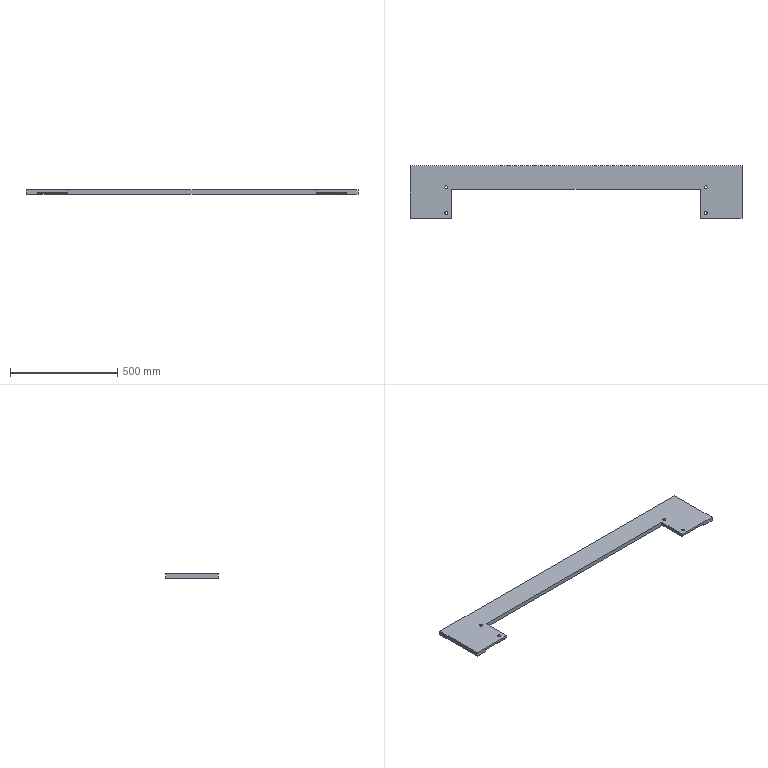Part | SolidWorks | features BaseBody 1 | 1 solid | 32 faces | box 1550 x 247 x 20 mm | volume 4227971 mm3 | plane 20 | cylinder 12 | commonest cylinder face diameters 14 x8 10 x4
STEP:
#1=CARTESIAN_POINT('',(612.,23.,20.));
#2=VERTEX_POINT('',#1);
#3=CARTESIAN_POINT('',(598.,23.,20.));
#4=VERTEX_POINT('',#3);
#5=CARTESIAN_POINT('',(605.,23.,20.));
#6=DIRECTION('',(0.,0.,-1.));
#7=DIRECTION('',(-1.,0.,0.));
#8=AXIS2_PLACEMENT_3D('',#5,#6,#7);
#9=CIRCLE('',#8,7.);
#10=EDGE_CURVE('',#2,#4,#9,.T.);
#11=ORIENTED_EDGE('',*,*,#10,.F.);
#12=CARTESIAN_POINT('',(612.,23.,5.));
#13=VERTEX_POINT('',#12);
#14=CARTESIAN_POINT('',(612.,23.,5.));
#15=DIRECTION('',(0.,0.,-1.));
#16=VECTOR('',#15,1000.);
#17=LINE('',#14,#16);
#18=EDGE_CURVE('',#2,#13,#17,.T.);
#19=ORIENTED_EDGE('',*,*,#18,.T.);
#20=CARTESIAN_POINT('',(598.,23.,5.));
#21=VERTEX_POINT('',#20);
#22=CARTESIAN_POINT('',(605.,23.,5.));
#23=DIRECTION('',(0.,0.,-1.));
#24=DIRECTION('',(-1.,0.,0.));
#25=AXIS2_PLACEMENT_3D('',#22,#23,#24);
#26=CIRCLE('',#25,7.);
#27=EDGE_CURVE('',#13,#21,#26,.T.);
#28=ORIENTED_EDGE('',*,*,#27,.T.);
#29=CARTESIAN_POINT('',(598.,23.,5.));
#30=DIRECTION('',(0.,0.,-1.));
#31=VECTOR('',#30,1000.);
#32=LINE('',#29,#31);
#33=EDGE_CURVE('',#4,#21,#32,.T.);
#34=ORIENTED_EDGE('',*,*,#33,.F.);
#35=EDGE_LOOP('',(#11,#19,#28,#34));
#36=FACE_OUTER_BOUND('',#35,.T.);
#37=CARTESIAN_POINT('',(605.,23.,5.));
#38=DIRECTION('',(0.,0.,-1.));
#39=DIRECTION('',(-1.,0.,0.));
#40=AXIS2_PLACEMENT_3D('',#37,#38,#39);
#41=CYLINDRICAL_SURFACE('',#40,7.);
#42=ADVANCED_FACE('',(#36),#41,.F.);
#43=CARTESIAN_POINT('',(612.,-97.,20.));
#44=VERTEX_POINT('',#43);
#45=CARTESIAN_POINT('',(598.,-97.,20.));
#46=VERTEX_POINT('',#45);
#47=CARTESIAN_POINT('',(605.,-97.,20.));
#48=DIRECTION('',(0.,0.,-1.));
#49=DIRECTION('',(-1.,0.,0.));
#50=AXIS2_PLACEMENT_3D('',#47,#48,#49);
#51=CIRCLE('',#50,7.);
#52=EDGE_CURVE('',#44,#46,#51,.T.);
#53=ORIENTED_EDGE('',*,*,#52,.F.);
#54=CARTESIAN_POINT('',(612.,-97.,5.));
#55=VERTEX_POINT('',#54);
#56=CARTESIAN_POINT('',(612.,-97.,5.));
#57=DIRECTION('',(0.,0.,-1.));
#58=VECTOR('',#57,1000.);
#59=LINE('',#56,#58);
#60=EDGE_CURVE('',#44,#55,#59,.T.);
#61=ORIENTED_EDGE('',*,*,#60,.T.);
#62=CARTESIAN_POINT('',(598.,-97.,5.));
#63=VERTEX_POINT('',#62);
#64=CARTESIAN_POINT('',(605.,-97.,5.));
#65=DIRECTION('',(0.,0.,-1.));
#66=DIRECTION('',(-1.,0.,0.));
#67=AXIS2_PLACEMENT_3D('',#64,#65,#66);
#68=CIRCLE('',#67,7.);
#69=EDGE_CURVE('',#55,#63,#68,.T.);
#70=ORIENTED_EDGE('',*,*,#69,.T.);
#71=CARTESIAN_POINT('',(598.,-97.,5.));
#72=DIRECTION('',(0.,0.,-1.));
#73=VECTOR('',#72,1000.);
#74=LINE('',#71,#73);
#75=EDGE_CURVE('',#46,#63,#74,.T.);
#76=ORIENTED_EDGE('',*,*,#75,.F.);
#77=EDGE_LOOP('',(#53,#61,#70,#76));
#78=FACE_OUTER_BOUND('',#77,.T.);
#79=CARTESIAN_POINT('',(605.,-97.,5.));
#80=DIRECTION('',(0.,0.,-1.));
#81=DIRECTION('',(-1.,0.,0.));
#82=AXIS2_PLACEMENT_3D('',#79,#80,#81);
#83=CYLINDRICAL_SURFACE('',#82,7.);
#84=ADVANCED_FACE('',(#78),#83,.F.);
#85=CARTESIAN_POINT('',(-598.,-97.,20.));
#86=VERTEX_POINT('',#85);
#87=CARTESIAN_POINT('',(-612.,-97.,20.));
#88=VERTEX_POINT('',#87);
#89=CARTESIAN_POINT('',(-605.,-97.,20.));
#90=DIRECTION('',(0.,0.,-1.));
#91=DIRECTION('',(-1.,0.,0.));
#92=AXIS2_PLACEMENT_3D('',#89,#90,#91);
#93=CIRCLE('',#92,7.);
#94=EDGE_CURVE('',#86,#88,#93,.T.);
#95=ORIENTED_EDGE('',*,*,#94,.F.);
#96=CARTESIAN_POINT('',(-598.,-97.,5.));
#97=VERTEX_POINT('',#96);
#98=CARTESIAN_POINT('',(-598.,-97.,5.));
#99=DIRECTION('',(0.,0.,-1.));
#100=VECTOR('',#99,1000.);
#101=LINE('',#98,#100);
#102=EDGE_CURVE('',#86,#97,#101,.T.);
#103=ORIENTED_EDGE('',*,*,#102,.T.);
#104=CARTESIAN_POINT('',(-612.,-97.,5.));
#105=VERTEX_POINT('',#104);
#106=CARTESIAN_POINT('',(-605.,-97.,5.));
#107=DIRECTION('',(0.,0.,-1.));
#108=DIRECTION('',(-1.,0.,0.));
#109=AXIS2_PLACEMENT_3D('',#106,#107,#108);
#110=CIRCLE('',#109,7.);
#111=EDGE_CURVE('',#97,#105,#110,.T.);
#112=ORIENTED_EDGE('',*,*,#111,.T.);
#113=CARTESIAN_POINT('',(-612.,-97.,5.));
#114=DIRECTION('',(0.,0.,-1.));
#115=VECTOR('',#114,1000.);
#116=LINE('',#113,#115);
#117=EDGE_CURVE('',#88,#105,#116,.T.);
#118=ORIENTED_EDGE('',*,*,#117,.F.);
#119=EDGE_LOOP('',(#95,#103,#112,#118));
#120=FACE_OUTER_BOUND('',#119,.T.);
#121=CARTESIAN_POINT('',(-605.,-97.,5.));
#122=DIRECTION('',(0.,0.,-1.));
#123=DIRECTION('',(-1.,0.,0.));
#124=AXIS2_PLACEMENT_3D('',#121,#122,#123);
#125=CYLINDRICAL_SURFACE('',#124,7.);
#126=ADVANCED_FACE('',(#120),#125,.F.);
#127=CARTESIAN_POINT('',(-598.,23.,20.));
#128=VERTEX_POINT('',#127);
#129=CARTESIAN_POINT('',(-612.,23.,20.));
#130=VERTEX_POINT('',#129);
#131=CARTESIAN_POINT('',(-605.,23.,20.));
#132=DIRECTION('',(0.,0.,-1.));
#133=DIRECTION('',(-1.,0.,0.));
#134=AXIS2_PLACEMENT_3D('',#131,#132,#133);
#135=CIRCLE('',#134,7.);
#136=EDGE_CURVE('',#128,#130,#135,.T.);
#137=ORIENTED_EDGE('',*,*,#136,.F.);
#138=CARTESIAN_POINT('',(-598.,23.,5.));
#139=VERTEX_POINT('',#138);
#140=CARTESIAN_POINT('',(-598.,23.,5.));
#141=DIRECTION('',(0.,0.,-1.));
#142=VECTOR('',#141,1000.);
#143=LINE('',#140,#142);
#144=EDGE_CURVE('',#128,#139,#143,.T.);
#145=ORIENTED_EDGE('',*,*,#144,.T.);
#146=CARTESIAN_POINT('',(-612.,23.,5.));
#147=VERTEX_POINT('',#146);
#148=CARTESIAN_POINT('',(-605.,23.,5.));
#149=DIRECTION('',(0.,0.,-1.));
#150=DIRECTION('',(-1.,0.,0.));
#151=AXIS2_PLACEMENT_3D('',#148,#149,#150);
#152=CIRCLE('',#151,7.);
#153=EDGE_CURVE('',#139,#147,#152,.T.);
#154=ORIENTED_EDGE('',*,*,#153,.T.);
#155=CARTESIAN_POINT('',(-612.,23.,5.));
#156=DIRECTION('',(0.,0.,-1.));
#157=VECTOR('',#156,1000.);
#158=LINE('',#155,#157);
#159=EDGE_CURVE('',#130,#147,#158,.T.);
#160=ORIENTED_EDGE('',*,*,#159,.F.);
#161=EDGE_LOOP('',(#137,#145,#154,#160));
#162=FACE_OUTER_BOUND('',#161,.T.);
#163=CARTESIAN_POINT('',(-605.,23.,5.));
#164=DIRECTION('',(0.,0.,-1.));
#165=DIRECTION('',(-1.,0.,0.));
#166=AXIS2_PLACEMENT_3D('',#163,#164,#165);
#167=CYLINDRICAL_SURFACE('',#166,7.);
#168=ADVANCED_FACE('',(#162),#167,.F.);
#169=CARTESIAN_POINT('',(580.,-117.,5.));
#170=VERTEX_POINT('',#169);
#171=CARTESIAN_POINT('',(580.,15.,5.));
#172=VERTEX_POINT('',#171);
#173=CARTESIAN_POINT('',(580.,-122.,5.));
#174=DIRECTION('',(0.,1.,0.));
#175=VECTOR('',#174,1000.);
#176=LINE('',#173,#175);
#177=EDGE_CURVE('',#170,#172,#176,.T.);
#178=ORIENTED_EDGE('',*,*,#177,.F.);
#179=CARTESIAN_POINT('',(580.,-122.,10.));
#180=VERTEX_POINT('',#179);
#181=CARTESIAN_POINT('',(580.,-117.,5.));
#182=DIRECTION('',(0.,-0.7071,0.7071));
#183=VECTOR('',#182,1000.);
#184=LINE('',#181,#183);
#185=EDGE_CURVE('',#170,#180,#184,.T.);
#186=ORIENTED_EDGE('',*,*,#185,.T.);
#187=CARTESIAN_POINT('',(580.,-122.,20.));
#188=VERTEX_POINT('',#187);
#189=CARTESIAN_POINT('',(580.,-122.,20.));
#190=DIRECTION('',(0.,0.,-1.));
#191=VECTOR('',#190,1000.);
#192=LINE('',#189,#191);
#193=EDGE_CURVE('',#188,#180,#192,.T.);
#194=ORIENTED_EDGE('',*,*,#193,.F.);
#195=CARTESIAN_POINT('',(580.,15.,20.));
#196=VERTEX_POINT('',#195);
#197=CARTESIAN_POINT('',(580.,15.,20.));
#198=DIRECTION('',(0.,-1.,0.));
#199=VECTOR('',#198,1000.);
#200=LINE('',#197,#199);
#201=EDGE_CURVE('',#196,#188,#200,.T.);
#202=ORIENTED_EDGE('',*,*,#201,.F.);
#203=CARTESIAN_POINT('',(580.,15.,20.));
#204=DIRECTION('',(0.,0.,-1.));
#205=VECTOR('',#204,1000.);
#206=LINE('',#203,#205);
#207=EDGE_CURVE('',#196,#172,#206,.T.);
#208=ORIENTED_EDGE('',*,*,#207,.T.);
#209=EDGE_LOOP('',(#178,#186,#194,#202,#208));
#210=FACE_OUTER_BOUND('',#209,.T.);
#211=CARTESIAN_POINT('',(580.,15.,20.));
#212=DIRECTION('',(1.,0.,0.));
#213=DIRECTION('',(0.,0.,-1.));
#214=AXIS2_PLACEMENT_3D('',#211,#212,#213);
#215=PLANE('',#214);
#216=ADVANCED_FACE('',(#210),#215,.F.);
#217=CARTESIAN_POINT('',(605.,23.,20.));
#218=DIRECTION('',(0.,0.,-1.));
#219=DIRECTION('',(-1.,0.,0.));
#220=AXIS2_PLACEMENT_3D('',#217,#218,#219);
#221=CIRCLE('',#220,7.);
#222=EDGE_CURVE('',#4,#2,#221,.T.);
#223=ORIENTED_EDGE('',*,*,#222,.T.);
#224=ORIENTED_EDGE('',*,*,#10,.T.);
#225=EDGE_LOOP('',(#223,#224));
#226=FACE_BOUND('',#225,.T.);
#227=CARTESIAN_POINT('',(605.,-97.,20.));
#228=DIRECTION('',(0.,0.,-1.));
#229=DIRECTION('',(-1.,0.,0.));
#230=AXIS2_PLACEMENT_3D('',#227,#228,#229);
#231=CIRCLE('',#230,7.);
#232=EDGE_CURVE('',#46,#44,#231,.T.);
#233=ORIENTED_EDGE('',*,*,#232,.T.);
#234=ORIENTED_EDGE('',*,*,#52,.T.);
#235=EDGE_LOOP('',(#233,#234));
#236=FACE_BOUND('',#235,.T.);
#237=CARTESIAN_POINT('',(-605.,-97.,20.));
#238=DIRECTION('',(0.,0.,-1.));
#239=DIRECTION('',(-1.,0.,0.));
#240=AXIS2_PLACEMENT_3D('',#237,#238,#239);
#241=CIRCLE('',#240,7.);
#242=EDGE_CURVE('',#88,#86,#241,.T.);
#243=ORIENTED_EDGE('',*,*,#242,.T.);
#244=ORIENTED_EDGE('',*,*,#94,.T.);
#245=EDGE_LOOP('',(#243,#244));
#246=FACE_BOUND('',#245,.T.);
#247=CARTESIAN_POINT('',(-605.,23.,20.));
#248=DIRECTION('',(0.,0.,-1.));
#249=DIRECTION('',(-1.,0.,0.));
#250=AXIS2_PLACEMENT_3D('',#247,#248,#249);
#251=CIRCLE('',#250,7.);
#252=EDGE_CURVE('',#130,#128,#251,.T.);
#253=ORIENTED_EDGE('',*,*,#252,.T.);
#254=ORIENTED_EDGE('',*,*,#136,.T.);
#255=EDGE_LOOP('',(#253,#254));
#256=FACE_BOUND('',#255,.T.);
#257=CARTESIAN_POINT('',(775.,-122.,20.));
#258=VERTEX_POINT('',#257);
#259=CARTESIAN_POINT('',(0.,-122.,20.));
#260=DIRECTION('',(-1.,0.,0.));
#261=VECTOR('',#260,1000.);
#262=LINE('',#259,#261);
#263=EDGE_CURVE('',#258,#188,#262,.T.);
#264=ORIENTED_EDGE('',*,*,#263,.F.);
#265=CARTESIAN_POINT('',(775.,125.,20.));
#266=VERTEX_POINT('',#265);
#267=CARTESIAN_POINT('',(775.,125.,20.));
#268=DIRECTION('',(0.,1.,0.));
#269=VECTOR('',#268,1000.);
#270=LINE('',#267,#269);
#271=EDGE_CURVE('',#258,#266,#270,.T.);
#272=ORIENTED_EDGE('',*,*,#271,.T.);
#273=CARTESIAN_POINT('',(-775.,125.,20.));
#274=VERTEX_POINT('',#273);
#275=CARTESIAN_POINT('',(-775.,125.,20.));
#276=DIRECTION('',(-1.,0.,0.));
#277=VECTOR('',#276,1000.);
#278=LINE('',#275,#277);
#279=EDGE_CURVE('',#266,#274,#278,.T.);
#280=ORIENTED_EDGE('',*,*,#279,.T.);
#281=CARTESIAN_POINT('',(-775.,-122.,20.));
#282=VERTEX_POINT('',#281);
#283=CARTESIAN_POINT('',(-775.,125.,20.));
#284=DIRECTION('',(0.,-1.,0.));
#285=VECTOR('',#284,1000.);
#286=LINE('',#283,#285);
#287=EDGE_CURVE('',#274,#282,#286,.T.);
#288=ORIENTED_EDGE('',*,*,#287,.T.);
#289=CARTESIAN_POINT('',(-580.,-122.,20.));
#290=VERTEX_POINT('',#289);
#291=CARTESIAN_POINT('',(0.,-122.,20.));
#292=DIRECTION('',(-1.,0.,0.));
#293=VECTOR('',#292,1000.);
#294=LINE('',#291,#293);
#295=EDGE_CURVE('',#290,#282,#294,.T.);
#296=ORIENTED_EDGE('',*,*,#295,.F.);
#297=CARTESIAN_POINT('',(-580.,15.,20.));
#298=VERTEX_POINT('',#297);
#299=CARTESIAN_POINT('',(-580.,15.,20.));
#300=DIRECTION('',(0.,1.,0.));
#301=VECTOR('',#300,1000.);
#302=LINE('',#299,#301);
#303=EDGE_CURVE('',#290,#298,#302,.T.);
#304=ORIENTED_EDGE('',*,*,#303,.T.);
#305=CARTESIAN_POINT('',(-580.,15.,20.));
#306=DIRECTION('',(1.,0.,0.));
#307=VECTOR('',#306,1000.);
#308=LINE('',#305,#307);
#309=EDGE_CURVE('',#298,#196,#308,.T.);
#310=ORIENTED_EDGE('',*,*,#309,.T.);
#311=ORIENTED_EDGE('',*,*,#201,.T.);
#312=EDGE_LOOP('',(#264,#272,#280,#288,#296,#304,#310,#311));
#313=FACE_OUTER_BOUND('',#312,.T.);
#314=CARTESIAN_POINT('',(0.,0.,20.));
#315=DIRECTION('',(0.,0.,-1.));
#316=DIRECTION('',(-1.,0.,0.));
#317=AXIS2_PLACEMENT_3D('',#314,#315,#316);
#318=PLANE('',#317);
#319=ADVANCED_FACE('',(#226,#236,#246,#256,#313),#318,.F.);
#320=CARTESIAN_POINT('',(-720.,-122.,0.));
#321=VERTEX_POINT('',#320);
#322=CARTESIAN_POINT('',(-720.,43.,0.));
#323=VERTEX_POINT('',#322);
#324=CARTESIAN_POINT('',(-720.,-122.,0.));
#325=DIRECTION('',(0.,1.,0.));
#326=VECTOR('',#325,1000.);
#327=LINE('',#324,#326);
#328=EDGE_CURVE('',#321,#323,#327,.T.);
#329=ORIENTED_EDGE('',*,*,#328,.F.);
#330=CARTESIAN_POINT('',(-775.,-122.,0.));
#331=VERTEX_POINT('',#330);
#332=CARTESIAN_POINT('',(-775.,-122.,0.));
#333=DIRECTION('',(1.,0.,0.));
#334=VECTOR('',#333,1000.);
#335=LINE('',#332,#334);
#336=EDGE_CURVE('',#331,#321,#335,.T.);
#337=ORIENTED_EDGE('',*,*,#336,.F.);
#338=CARTESIAN_POINT('',(-775.,125.,0.));
#339=VERTEX_POINT('',#338);
#340=CARTESIAN_POINT('',(-775.,125.,0.));
#341=DIRECTION('',(0.,-1.,0.));
#342=VECTOR('',#341,1000.);
#343=LINE('',#340,#342);
#344=EDGE_CURVE('',#339,#331,#343,.T.);
#345=ORIENTED_EDGE('',*,*,#344,.F.);
#346=CARTESIAN_POINT('',(775.,125.,0.));
#347=VERTEX_POINT('',#346);
#348=CARTESIAN_POINT('',(-775.,125.,0.));
#349=DIRECTION('',(-1.,0.,0.));
#350=VECTOR('',#349,1000.);
#351=LINE('',#348,#350);
#352=EDGE_CURVE('',#347,#339,#351,.T.);
#353=ORIENTED_EDGE('',*,*,#352,.F.);
#354=CARTESIAN_POINT('',(775.,-122.,0.));
#355=VERTEX_POINT('',#354);
#356=CARTESIAN_POINT('',(775.,125.,0.));
#357=DIRECTION('',(0.,1.,0.));
#358=VECTOR('',#357,1000.);
#359=LINE('',#356,#358);
#360=EDGE_CURVE('',#355,#347,#359,.T.);
#361=ORIENTED_EDGE('',*,*,#360,.F.);
#362=CARTESIAN_POINT('',(720.,-122.,0.));
#363=VERTEX_POINT('',#362);
#364=CARTESIAN_POINT('',(580.,-122.,0.));
#365=DIRECTION('',(1.,0.,0.));
#366=VECTOR('',#365,1000.);
#367=LINE('',#364,#366);
#368=EDGE_CURVE('',#363,#355,#367,.T.);
#369=ORIENTED_EDGE('',*,*,#368,.F.);
#370=CARTESIAN_POINT('',(720.,43.,0.));
#371=VERTEX_POINT('',#370);
#372=CARTESIAN_POINT('',(720.,-122.,0.));
#373=DIRECTION('',(0.,-1.,0.));
#374=VECTOR('',#373,1000.);
#375=LINE('',#372,#374);
#376=EDGE_CURVE('',#371,#363,#375,.T.);
#377=ORIENTED_EDGE('',*,*,#376,.F.);
#378=CARTESIAN_POINT('',(715.,48.,0.));
#379=VERTEX_POINT('',#378);
#380=CARTESIAN_POINT('',(715.,43.,0.));
#381=DIRECTION('',(0.,0.,-1.));
#382=DIRECTION('',(-1.,0.,0.));
#383=AXIS2_PLACEMENT_3D('',#380,#381,#382);
#384=CIRCLE('',#383,5.);
#385=EDGE_CURVE('',#379,#371,#384,.T.);
#386=ORIENTED_EDGE('',*,*,#385,.F.);
#387=CARTESIAN_POINT('',(585.,48.,0.));
#388=VERTEX_POINT('',#387);
#389=CARTESIAN_POINT('',(585.,48.,0.));
#390=DIRECTION('',(1.,0.,0.));
#391=VECTOR('',#390,1000.);
#392=LINE('',#389,#391);
#393=EDGE_CURVE('',#388,#379,#392,.T.);
#394=ORIENTED_EDGE('',*,*,#393,.F.);
#395=CARTESIAN_POINT('',(580.,43.,0.));
#396=VERTEX_POINT('',#395);
#397=CARTESIAN_POINT('',(585.,43.,0.));
#398=DIRECTION('',(0.,0.,-1.));
#399=DIRECTION('',(-1.,0.,0.));
#400=AXIS2_PLACEMENT_3D('',#397,#398,#399);
#401=CIRCLE('',#400,5.);
#402=EDGE_CURVE('',#396,#388,#401,.T.);
#403=ORIENTED_EDGE('',*,*,#402,.F.);
#404=CARTESIAN_POINT('',(580.,15.,0.));
#405=VERTEX_POINT('',#404);
#406=CARTESIAN_POINT('',(580.,-122.,0.));
#407=DIRECTION('',(0.,1.,0.));
#408=VECTOR('',#407,1000.);
#409=LINE('',#406,#408);
#410=EDGE_CURVE('',#405,#396,#409,.T.);
#411=ORIENTED_EDGE('',*,*,#410,.F.);
#412=CARTESIAN_POINT('',(-580.,15.,0.));
#413=VERTEX_POINT('',#412);
#414=CARTESIAN_POINT('',(-580.,15.,0.));
#415=DIRECTION('',(1.,0.,0.));
#416=VECTOR('',#415,1000.);
#417=LINE('',#414,#416);
#418=EDGE_CURVE('',#413,#405,#417,.T.);
#419=ORIENTED_EDGE('',*,*,#418,.F.);
#420=CARTESIAN_POINT('',(-580.,43.,0.));
#421=VERTEX_POINT('',#420);
#422=CARTESIAN_POINT('',(-580.,-122.,0.));
#423=DIRECTION('',(0.,-1.,0.));
#424=VECTOR('',#423,1000.);
#425=LINE('',#422,#424);
#426=EDGE_CURVE('',#421,#413,#425,.T.);
#427=ORIENTED_EDGE('',*,*,#426,.F.);
#428=CARTESIAN_POINT('',(-585.,48.,0.));
#429=VERTEX_POINT('',#428);
#430=CARTESIAN_POINT('',(-585.,43.,0.));
#431=DIRECTION('',(0.,0.,-1.));
#432=DIRECTION('',(1.,0.,0.));
#433=AXIS2_PLACEMENT_3D('',#430,#431,#432);
#434=CIRCLE('',#433,5.);
#435=EDGE_CURVE('',#429,#421,#434,.T.);
#436=ORIENTED_EDGE('',*,*,#435,.F.);
#437=CARTESIAN_POINT('',(-715.,48.,0.));
#438=VERTEX_POINT('',#437);
#439=CARTESIAN_POINT('',(-585.,48.,0.));
#440=DIRECTION('',(1.,0.,0.));
#441=VECTOR('',#440,1000.);
#442=LINE('',#439,#441);
#443=EDGE_CURVE('',#438,#429,#442,.T.);
#444=ORIENTED_EDGE('',*,*,#443,.F.);
#445=CARTESIAN_POINT('',(-715.,43.,0.));
#446=DIRECTION('',(0.,0.,-1.));
#447=DIRECTION('',(1.,0.,0.));
#448=AXIS2_PLACEMENT_3D('',#445,#446,#447);
#449=CIRCLE('',#448,5.);
#450=EDGE_CURVE('',#323,#438,#449,.T.);
#451=ORIENTED_EDGE('',*,*,#450,.F.);
#452=EDGE_LOOP('',(#329,#337,#345,#353,#361,#369,#377,#386,#394,#403,#411,#419,#427,#436,#444,#451));
#453=FACE_OUTER_BOUND('',#452,.T.);
#454=CARTESIAN_POINT('',(0.,0.,0.));
#455=DIRECTION('',(0.,0.,-1.));
#456=DIRECTION('',(-1.,0.,0.));
#457=AXIS2_PLACEMENT_3D('',#454,#455,#456);
#458=PLANE('',#457);
#459=ADVANCED_FACE('',(#453),#458,.T.);
#460=CARTESIAN_POINT('',(775.,-122.,170.));
#461=DIRECTION('',(0.,0.,1.));
#462=VECTOR('',#461,1000.);
#463=LINE('',#460,#462);
#464=EDGE_CURVE('',#355,#258,#463,.T.);
#465=ORIENTED_EDGE('',*,*,#464,.F.);
#466=ORIENTED_EDGE('',*,*,#360,.T.);
#467=CARTESIAN_POINT('',(775.,125.,20.));
#468=DIRECTION('',(0.,0.,-1.));
#469=VECTOR('',#468,1000.);
#470=LINE('',#467,#469);
#471=EDGE_CURVE('',#266,#347,#470,.T.);
#472=ORIENTED_EDGE('',*,*,#471,.F.);
#473=ORIENTED_EDGE('',*,*,#271,.F.);
#474=EDGE_LOOP('',(#465,#466,#472,#473));
#475=FACE_OUTER_BOUND('',#474,.T.);
#476=CARTESIAN_POINT('',(775.,125.,20.));
#477=DIRECTION('',(-1.,0.,0.));
#478=DIRECTION('',(0.,0.,1.));
#479=AXIS2_PLACEMENT_3D('',#476,#477,#478);
#480=PLANE('',#479);
#481=ADVANCED_FACE('',(#475),#480,.F.);
#482=CARTESIAN_POINT('',(-775.,-122.,170.));
#483=DIRECTION('',(0.,0.,-1.));
#484=VECTOR('',#483,1000.);
#485=LINE('',#482,#484);
#486=EDGE_CURVE('',#282,#331,#485,.T.);
#487=ORIENTED_EDGE('',*,*,#486,.F.);
#488=ORIENTED_EDGE('',*,*,#287,.F.);
#489=CARTESIAN_POINT('',(-775.,125.,20.));
#490=DIRECTION('',(0.,0.,-1.));
#491=VECTOR('',#490,1000.);
#492=LINE('',#489,#491);
#493=EDGE_CURVE('',#274,#339,#492,.T.);
#494=ORIENTED_EDGE('',*,*,#493,.T.);
#495=ORIENTED_EDGE('',*,*,#344,.T.);
#496=EDGE_LOOP('',(#487,#488,#494,#495));
#497=FACE_OUTER_BOUND('',#496,.T.);
#498=CARTESIAN_POINT('',(-775.,125.,20.));
#499=DIRECTION('',(1.,0.,0.));
#500=DIRECTION('',(0.,0.,-1.));
#501=AXIS2_PLACEMENT_3D('',#498,#499,#500);
#502=PLANE('',#501);
#503=ADVANCED_FACE('',(#497),#502,.F.);
#504=CARTESIAN_POINT('',(-580.,-122.,10.));
#505=VERTEX_POINT('',#504);
#506=CARTESIAN_POINT('',(-580.,-122.,170.));
#507=DIRECTION('',(0.,0.,1.));
#508=VECTOR('',#507,1000.);
#509=LINE('',#506,#508);
#510=EDGE_CURVE('',#505,#290,#509,.T.);
#511=ORIENTED_EDGE('',*,*,#510,.F.);
#512=CARTESIAN_POINT('',(-580.,-117.,5.));
#513=VERTEX_POINT('',#512);
#514=CARTESIAN_POINT('',(-580.,-117.,5.));
#515=DIRECTION('',(0.,0.7071,-0.7071));
#516=VECTOR('',#515,1000.);
#517=LINE('',#514,#516);
#518=EDGE_CURVE('',#505,#513,#517,.T.);
#519=ORIENTED_EDGE('',*,*,#518,.T.);
#520=CARTESIAN_POINT('',(-580.,15.,5.));
#521=VERTEX_POINT('',#520);
#522=CARTESIAN_POINT('',(-580.,-122.,5.));
#523=DIRECTION('',(0.,-1.,0.));
#524=VECTOR('',#523,1000.);
#525=LINE('',#522,#524);
#526=EDGE_CURVE('',#521,#513,#525,.T.);
#527=ORIENTED_EDGE('',*,*,#526,.F.);
#528=CARTESIAN_POINT('',(-580.,15.,20.));
#529=DIRECTION('',(0.,0.,-1.));
#530=VECTOR('',#529,1000.);
#531=LINE('',#528,#530);
#532=EDGE_CURVE('',#298,#521,#531,.T.);
#533=ORIENTED_EDGE('',*,*,#532,.F.);
#534=ORIENTED_EDGE('',*,*,#303,.F.);
#535=EDGE_LOOP('',(#511,#519,#527,#533,#534));
#536=FACE_OUTER_BOUND('',#535,.T.);
#537=CARTESIAN_POINT('',(-580.,15.,20.));
#538=DIRECTION('',(-1.,0.,0.));
#539=DIRECTION('',(0.,0.,1.));
#540=AXIS2_PLACEMENT_3D('',#537,#538,#539);
#541=PLANE('',#540);
#542=ADVANCED_FACE('',(#536),#541,.F.);
#543=ORIENTED_EDGE('',*,*,#352,.T.);
#544=ORIENTED_EDGE('',*,*,#493,.F.);
#545=ORIENTED_EDGE('',*,*,#279,.F.);
#546=ORIENTED_EDGE('',*,*,#471,.T.);
#547=EDGE_LOOP('',(#543,#544,#545,#546));
#548=FACE_OUTER_BOUND('',#547,.T.);
#549=CARTESIAN_POINT('',(-775.,125.,20.));
#550=DIRECTION('',(0.,-1.,0.));
#551=DIRECTION('',(0.,0.,-1.));
#552=AXIS2_PLACEMENT_3D('',#549,#550,#551);
#553=PLANE('',#552);
#554=ADVANCED_FACE('',(#548),#553,.F.);
#555=ORIENTED_EDGE('',*,*,#418,.T.);
#556=CARTESIAN_POINT('',(580.,15.,20.));
#557=DIRECTION('',(0.,0.,1.));
#558=VECTOR('',#557,1000.);
#559=LINE('',#556,#558);
#560=EDGE_CURVE('',#405,#172,#559,.T.);
#561=ORIENTED_EDGE('',*,*,#560,.T.);
#562=ORIENTED_EDGE('',*,*,#207,.F.);
#563=ORIENTED_EDGE('',*,*,#309,.F.);
#564=ORIENTED_EDGE('',*,*,#532,.T.);
#565=CARTESIAN_POINT('',(-580.,15.,20.));
#566=DIRECTION('',(0.,0.,-1.));
#567=VECTOR('',#566,1000.);
#568=LINE('',#565,#567);
#569=EDGE_CURVE('',#521,#413,#568,.T.);
#570=ORIENTED_EDGE('',*,*,#569,.T.);
#571=EDGE_LOOP('',(#555,#561,#562,#563,#564,#570));
#572=FACE_OUTER_BOUND('',#571,.T.);
#573=CARTESIAN_POINT('',(-580.,15.,20.));
#574=DIRECTION('',(0.,1.,0.));
#575=DIRECTION('',(0.,0.,1.));
#576=AXIS2_PLACEMENT_3D('',#573,#574,#575);
#577=PLANE('',#576);
#578=ADVANCED_FACE('',(#572),#577,.F.);
#579=CARTESIAN_POINT('',(-720.,-122.,10.));
#580=VERTEX_POINT('',#579);
#581=CARTESIAN_POINT('',(-720.,-122.,5.));
#582=DIRECTION('',(0.,0.,-1.));
#583=VECTOR('',#582,1000.);
#584=LINE('',#581,#583);
#585=EDGE_CURVE('',#580,#321,#584,.T.);
#586=ORIENTED_EDGE('',*,*,#585,.F.);
#587=CARTESIAN_POINT('',(-580.,-122.,10.));
#588=DIRECTION('',(1.,0.,0.));
#589=VECTOR('',#588,1000.);
#590=LINE('',#587,#589);
#591=EDGE_CURVE('',#580,#505,#590,.T.);
#592=ORIENTED_EDGE('',*,*,#591,.T.);
#593=ORIENTED_EDGE('',*,*,#510,.T.);
#594=ORIENTED_EDGE('',*,*,#295,.T.);
#595=ORIENTED_EDGE('',*,*,#486,.T.);
#596=ORIENTED_EDGE('',*,*,#336,.T.);
#597=EDGE_LOOP('',(#586,#592,#593,#594,#595,#596));
#598=FACE_OUTER_BOUND('',#597,.T.);
#599=CARTESIAN_POINT('',(0.,-122.,85.));
#600=DIRECTION('',(0.,-1.,0.));
#601=DIRECTION('',(0.,0.,-1.));
#602=AXIS2_PLACEMENT_3D('',#599,#600,#601);
#603=PLANE('',#602);
#604=ADVANCED_FACE('',(#598),#603,.T.);
#605=ORIENTED_EDGE('',*,*,#193,.T.);
#606=CARTESIAN_POINT('',(720.,-122.,10.));
#607=VERTEX_POINT('',#606);
#608=CARTESIAN_POINT('',(0.,-122.,10.));
#609=DIRECTION('',(1.,0.,0.));
#610=VECTOR('',#609,1000.);
#611=LINE('',#608,#610);
#612=EDGE_CURVE('',#180,#607,#611,.T.);
#613=ORIENTED_EDGE('',*,*,#612,.T.);
#614=CARTESIAN_POINT('',(720.,-122.,5.));
#615=DIRECTION('',(0.,0.,-1.));
#616=VECTOR('',#615,1000.);
#617=LINE('',#614,#616);
#618=EDGE_CURVE('',#607,#363,#617,.T.);
#619=ORIENTED_EDGE('',*,*,#618,.T.);
#620=ORIENTED_EDGE('',*,*,#368,.T.);
#621=ORIENTED_EDGE('',*,*,#464,.T.);
#622=ORIENTED_EDGE('',*,*,#263,.T.);
#623=EDGE_LOOP('',(#605,#613,#619,#620,#621,#622));
#624=FACE_OUTER_BOUND('',#623,.T.);
#625=CARTESIAN_POINT('',(0.,-122.,85.));
#626=DIRECTION('',(0.,-1.,0.));
#627=DIRECTION('',(0.,0.,-1.));
#628=AXIS2_PLACEMENT_3D('',#625,#626,#627);
#629=PLANE('',#628);
#630=ADVANCED_FACE('',(#624),#629,.T.);
#631=ORIENTED_EDGE('',*,*,#410,.T.);
#632=CARTESIAN_POINT('',(580.,43.,5.));
#633=VERTEX_POINT('',#632);
#634=CARTESIAN_POINT('',(580.,43.,5.));
#635=DIRECTION('',(0.,0.,-1.));
#636=VECTOR('',#635,1000.);
#637=LINE('',#634,#636);
#638=EDGE_CURVE('',#633,#396,#637,.T.);
#639=ORIENTED_EDGE('',*,*,#638,.F.);
#640=CARTESIAN_POINT('',(580.,-122.,5.));
#641=DIRECTION('',(0.,1.,0.));
#642=VECTOR('',#641,1000.);
#643=LINE('',#640,#642);
#644=EDGE_CURVE('',#172,#633,#643,.T.);
#645=ORIENTED_EDGE('',*,*,#644,.F.);
#646=ORIENTED_EDGE('',*,*,#560,.F.);
#647=EDGE_LOOP('',(#631,#639,#645,#646));
#648=FACE_OUTER_BOUND('',#647,.T.);
#649=CARTESIAN_POINT('',(580.,-122.,5.));
#650=DIRECTION('',(-1.,0.,0.));
#651=DIRECTION('',(0.,0.,1.));
#652=AXIS2_PLACEMENT_3D('',#649,#650,#651);
#653=PLANE('',#652);
#654=ADVANCED_FACE('',(#648),#653,.F.);
#655=ORIENTED_EDGE('',*,*,#376,.T.);
#656=ORIENTED_EDGE('',*,*,#618,.F.);
#657=CARTESIAN_POINT('',(720.,-117.,5.));
#658=VERTEX_POINT('',#657);
#659=CARTESIAN_POINT('',(720.,-119.5,7.5));
#660=DIRECTION('',(0.,0.7071,-0.7071));
#661=VECTOR('',#660,1000.);
#662=LINE('',#659,#661);
#663=EDGE_CURVE('',#607,#658,#662,.T.);
#664=ORIENTED_EDGE('',*,*,#663,.T.);
#665=CARTESIAN_POINT('',(720.,43.,5.));
#666=VERTEX_POINT('',#665);
#667=CARTESIAN_POINT('',(720.,-122.,5.));
#668=DIRECTION('',(0.,-1.,0.));
#669=VECTOR('',#668,1000.);
#670=LINE('',#667,#669);
#671=EDGE_CURVE('',#666,#658,#670,.T.);
#672=ORIENTED_EDGE('',*,*,#671,.F.);
#673=CARTESIAN_POINT('',(720.,43.,5.));
#674=DIRECTION('',(0.,0.,-1.));
#675=VECTOR('',#674,1000.);
#676=LINE('',#673,#675);
#677=EDGE_CURVE('',#666,#371,#676,.T.);
#678=ORIENTED_EDGE('',*,*,#677,.T.);
#679=EDGE_LOOP('',(#655,#656,#664,#672,#678));
#680=FACE_OUTER_BOUND('',#679,.T.);
#681=CARTESIAN_POINT('',(720.,-122.,5.));
#682=DIRECTION('',(1.,0.,0.));
#683=DIRECTION('',(0.,0.,-1.));
#684=AXIS2_PLACEMENT_3D('',#681,#682,#683);
#685=PLANE('',#684);
#686=ADVANCED_FACE('',(#680),#685,.F.);
#687=ORIENTED_EDGE('',*,*,#385,.T.);
#688=ORIENTED_EDGE('',*,*,#677,.F.);
#689=CARTESIAN_POINT('',(715.,48.,5.));
#690=VERTEX_POINT('',#689);
#691=CARTESIAN_POINT('',(715.,43.,5.));
#692=DIRECTION('',(0.,0.,-1.));
#693=DIRECTION('',(-1.,0.,0.));
#694=AXIS2_PLACEMENT_3D('',#691,#692,#693);
#695=CIRCLE('',#694,5.);
#696=EDGE_CURVE('',#690,#666,#695,.T.);
#697=ORIENTED_EDGE('',*,*,#696,.F.);
#698=CARTESIAN_POINT('',(715.,48.,5.));
#699=DIRECTION('',(0.,0.,-1.));
#700=VECTOR('',#699,1000.);
#701=LINE('',#698,#700);
#702=EDGE_CURVE('',#690,#379,#701,.T.);
#703=ORIENTED_EDGE('',*,*,#702,.T.);
#704=EDGE_LOOP('',(#687,#688,#697,#703));
#705=FACE_OUTER_BOUND('',#704,.T.);
#706=CARTESIAN_POINT('',(715.,43.,5.));
#707=DIRECTION('',(0.,0.,-1.));
#708=DIRECTION('',(-1.,0.,0.));
#709=AXIS2_PLACEMENT_3D('',#706,#707,#708);
#710=CYLINDRICAL_SURFACE('',#709,5.);
#711=ADVANCED_FACE('',(#705),#710,.F.);
#712=ORIENTED_EDGE('',*,*,#393,.T.);
#713=ORIENTED_EDGE('',*,*,#702,.F.);
#714=CARTESIAN_POINT('',(585.,48.,5.));
#715=VERTEX_POINT('',#714);
#716=CARTESIAN_POINT('',(585.,48.,5.));
#717=DIRECTION('',(1.,0.,0.));
#718=VECTOR('',#717,1000.);
#719=LINE('',#716,#718);
#720=EDGE_CURVE('',#715,#690,#719,.T.);
#721=ORIENTED_EDGE('',*,*,#720,.F.);
#722=CARTESIAN_POINT('',(585.,48.,5.));
#723=DIRECTION('',(0.,0.,-1.));
#724=VECTOR('',#723,1000.);
#725=LINE('',#722,#724);
#726=EDGE_CURVE('',#715,#388,#725,.T.);
#727=ORIENTED_EDGE('',*,*,#726,.T.);
#728=EDGE_LOOP('',(#712,#713,#721,#727));
#729=FACE_OUTER_BOUND('',#728,.T.);
#730=CARTESIAN_POINT('',(585.,48.,5.));
#731=DIRECTION('',(0.,1.,0.));
#732=DIRECTION('',(-1.,0.,0.));
#733=AXIS2_PLACEMENT_3D('',#730,#731,#732);
#734=PLANE('',#733);
#735=ADVANCED_FACE('',(#729),#734,.F.);
#736=ORIENTED_EDGE('',*,*,#402,.T.);
#737=ORIENTED_EDGE('',*,*,#726,.F.);
#738=CARTESIAN_POINT('',(585.,43.,5.));
#739=DIRECTION('',(0.,0.,-1.));
#740=DIRECTION('',(-1.,0.,0.));
#741=AXIS2_PLACEMENT_3D('',#738,#739,#740);
#742=CIRCLE('',#741,5.);
#743=EDGE_CURVE('',#633,#715,#742,.T.);
#744=ORIENTED_EDGE('',*,*,#743,.F.);
#745=ORIENTED_EDGE('',*,*,#638,.T.);
#746=EDGE_LOOP('',(#736,#737,#744,#745));
#747=FACE_OUTER_BOUND('',#746,.T.);
#748=CARTESIAN_POINT('',(585.,43.,5.));
#749=DIRECTION('',(0.,0.,-1.));
#750=DIRECTION('',(-1.,0.,0.));
#751=AXIS2_PLACEMENT_3D('',#748,#749,#750);
#752=CYLINDRICAL_SURFACE('',#751,5.);
#753=ADVANCED_FACE('',(#747),#752,.F.);
#754=CARTESIAN_POINT('',(605.,23.,5.));
#755=DIRECTION('',(0.,0.,-1.));
#756=DIRECTION('',(-1.,0.,0.));
#757=AXIS2_PLACEMENT_3D('',#754,#755,#756);
#758=CIRCLE('',#757,7.);
#759=EDGE_CURVE('',#21,#13,#758,.T.);
#760=ORIENTED_EDGE('',*,*,#759,.F.);
#761=ORIENTED_EDGE('',*,*,#27,.F.);
#762=EDGE_LOOP('',(#760,#761));
#763=FACE_BOUND('',#762,.T.);
#764=CARTESIAN_POINT('',(605.,-97.,5.));
#765=DIRECTION('',(0.,0.,-1.));
#766=DIRECTION('',(-1.,0.,0.));
#767=AXIS2_PLACEMENT_3D('',#764,#765,#766);
#768=CIRCLE('',#767,7.);
#769=EDGE_CURVE('',#63,#55,#768,.T.);
#770=ORIENTED_EDGE('',*,*,#769,.F.);
#771=ORIENTED_EDGE('',*,*,#69,.F.);
#772=EDGE_LOOP('',(#770,#771));
#773=FACE_BOUND('',#772,.T.);
#774=ORIENTED_EDGE('',*,*,#671,.T.);
#775=CARTESIAN_POINT('',(585.,-117.,5.));
#776=DIRECTION('',(-1.,0.,0.));
#777=VECTOR('',#776,1000.);
#778=LINE('',#775,#777);
#779=EDGE_CURVE('',#658,#170,#778,.T.);
#780=ORIENTED_EDGE('',*,*,#779,.T.);
#781=ORIENTED_EDGE('',*,*,#177,.T.);
#782=ORIENTED_EDGE('',*,*,#644,.T.);
#783=ORIENTED_EDGE('',*,*,#743,.T.);
#784=ORIENTED_EDGE('',*,*,#720,.T.);
#785=ORIENTED_EDGE('',*,*,#696,.T.);
#786=EDGE_LOOP('',(#774,#780,#781,#782,#783,#784,#785));
#787=FACE_OUTER_BOUND('',#786,.T.);
#788=CARTESIAN_POINT('',(585.,43.,5.));
#789=DIRECTION('',(0.,0.,-1.));
#790=DIRECTION('',(-1.,0.,0.));
#791=AXIS2_PLACEMENT_3D('',#788,#789,#790);
#792=PLANE('',#791);
#793=ADVANCED_FACE('',(#763,#773,#787),#792,.T.);
#794=CARTESIAN_POINT('',(-580.,43.,5.));
#795=VERTEX_POINT('',#794);
#796=CARTESIAN_POINT('',(-580.,-122.,5.));
#797=DIRECTION('',(0.,-1.,0.));
#798=VECTOR('',#797,1000.);
#799=LINE('',#796,#798);
#800=EDGE_CURVE('',#795,#521,#799,.T.);
#801=ORIENTED_EDGE('',*,*,#800,.F.);
#802=CARTESIAN_POINT('',(-580.,43.,5.));
#803=DIRECTION('',(0.,0.,-1.));
#804=VECTOR('',#803,1000.);
#805=LINE('',#802,#804);
#806=EDGE_CURVE('',#795,#421,#805,.T.);
#807=ORIENTED_EDGE('',*,*,#806,.T.);
#808=ORIENTED_EDGE('',*,*,#426,.T.);
#809=ORIENTED_EDGE('',*,*,#569,.F.);
#810=EDGE_LOOP('',(#801,#807,#808,#809));
#811=FACE_OUTER_BOUND('',#810,.T.);
#812=CARTESIAN_POINT('',(-580.,-122.,5.));
#813=DIRECTION('',(1.,0.,0.));
#814=DIRECTION('',(0.,0.,-1.));
#815=AXIS2_PLACEMENT_3D('',#812,#813,#814);
#816=PLANE('',#815);
#817=ADVANCED_FACE('',(#811),#816,.F.);
#818=ORIENTED_EDGE('',*,*,#450,.T.);
#819=CARTESIAN_POINT('',(-715.,48.,5.));
#820=VERTEX_POINT('',#819);
#821=CARTESIAN_POINT('',(-715.,48.,5.));
#822=DIRECTION('',(0.,0.,-1.));
#823=VECTOR('',#822,1000.);
#824=LINE('',#821,#823);
#825=EDGE_CURVE('',#820,#438,#824,.T.);
#826=ORIENTED_EDGE('',*,*,#825,.F.);
#827=CARTESIAN_POINT('',(-720.,43.,5.));
#828=VERTEX_POINT('',#827);
#829=CARTESIAN_POINT('',(-715.,43.,5.));
#830=DIRECTION('',(0.,0.,-1.));
#831=DIRECTION('',(1.,0.,0.));
#832=AXIS2_PLACEMENT_3D('',#829,#830,#831);
#833=CIRCLE('',#832,5.);
#834=EDGE_CURVE('',#828,#820,#833,.T.);
#835=ORIENTED_EDGE('',*,*,#834,.F.);
#836=CARTESIAN_POINT('',(-720.,43.,5.));
#837=DIRECTION('',(0.,0.,-1.));
#838=VECTOR('',#837,1000.);
#839=LINE('',#836,#838);
#840=EDGE_CURVE('',#828,#323,#839,.T.);
#841=ORIENTED_EDGE('',*,*,#840,.T.);
#842=EDGE_LOOP('',(#818,#826,#835,#841));
#843=FACE_OUTER_BOUND('',#842,.T.);
#844=CARTESIAN_POINT('',(-715.,43.,5.));
#845=DIRECTION('',(0.,0.,-1.));
#846=DIRECTION('',(-1.,0.,0.));
#847=AXIS2_PLACEMENT_3D('',#844,#845,#846);
#848=CYLINDRICAL_SURFACE('',#847,5.);
#849=ADVANCED_FACE('',(#843),#848,.F.);
#850=ORIENTED_EDGE('',*,*,#328,.T.);
#851=ORIENTED_EDGE('',*,*,#840,.F.);
#852=CARTESIAN_POINT('',(-720.,-117.,5.));
#853=VERTEX_POINT('',#852);
#854=CARTESIAN_POINT('',(-720.,-122.,5.));
#855=DIRECTION('',(0.,1.,0.));
#856=VECTOR('',#855,1000.);
#857=LINE('',#854,#856);
#858=EDGE_CURVE('',#853,#828,#857,.T.);
#859=ORIENTED_EDGE('',*,*,#858,.F.);
#860=CARTESIAN_POINT('',(-720.,-119.5,7.5));
#861=DIRECTION('',(0.,-0.7071,0.7071));
#862=VECTOR('',#861,1000.);
#863=LINE('',#860,#862);
#864=EDGE_CURVE('',#853,#580,#863,.T.);
#865=ORIENTED_EDGE('',*,*,#864,.T.);
#866=ORIENTED_EDGE('',*,*,#585,.T.);
#867=EDGE_LOOP('',(#850,#851,#859,#865,#866));
#868=FACE_OUTER_BOUND('',#867,.T.);
#869=CARTESIAN_POINT('',(-720.,-122.,5.));
#870=DIRECTION('',(-1.,0.,0.));
#871=DIRECTION('',(0.,0.,1.));
#872=AXIS2_PLACEMENT_3D('',#869,#870,#871);
#873=PLANE('',#872);
#874=ADVANCED_FACE('',(#868),#873,.F.);
#875=ORIENTED_EDGE('',*,*,#435,.T.);
#876=ORIENTED_EDGE('',*,*,#806,.F.);
#877=CARTESIAN_POINT('',(-585.,48.,5.));
#878=VERTEX_POINT('',#877);
#879=CARTESIAN_POINT('',(-585.,43.,5.));
#880=DIRECTION('',(0.,0.,-1.));
#881=DIRECTION('',(1.,0.,0.));
#882=AXIS2_PLACEMENT_3D('',#879,#880,#881);
#883=CIRCLE('',#882,5.);
#884=EDGE_CURVE('',#878,#795,#883,.T.);
#885=ORIENTED_EDGE('',*,*,#884,.F.);
#886=CARTESIAN_POINT('',(-585.,48.,5.));
#887=DIRECTION('',(0.,0.,-1.));
#888=VECTOR('',#887,1000.);
#889=LINE('',#886,#888);
#890=EDGE_CURVE('',#878,#429,#889,.T.);
#891=ORIENTED_EDGE('',*,*,#890,.T.);
#892=EDGE_LOOP('',(#875,#876,#885,#891));
#893=FACE_OUTER_BOUND('',#892,.T.);
#894=CARTESIAN_POINT('',(-585.,43.,5.));
#895=DIRECTION('',(0.,0.,-1.));
#896=DIRECTION('',(-1.,0.,0.));
#897=AXIS2_PLACEMENT_3D('',#894,#895,#896);
#898=CYLINDRICAL_SURFACE('',#897,5.);
#899=ADVANCED_FACE('',(#893),#898,.F.);
#900=ORIENTED_EDGE('',*,*,#443,.T.);
#901=ORIENTED_EDGE('',*,*,#890,.F.);
#902=CARTESIAN_POINT('',(-585.,48.,5.));
#903=DIRECTION('',(1.,0.,0.));
#904=VECTOR('',#903,1000.);
#905=LINE('',#902,#904);
#906=EDGE_CURVE('',#820,#878,#905,.T.);
#907=ORIENTED_EDGE('',*,*,#906,.F.);
#908=ORIENTED_EDGE('',*,*,#825,.T.);
#909=EDGE_LOOP('',(#900,#901,#907,#908));
#910=FACE_OUTER_BOUND('',#909,.T.);
#911=CARTESIAN_POINT('',(-585.,48.,5.));
#912=DIRECTION('',(0.,1.,0.));
#913=DIRECTION('',(-1.,0.,0.));
#914=AXIS2_PLACEMENT_3D('',#911,#912,#913);
#915=PLANE('',#914);
#916=ADVANCED_FACE('',(#910),#915,.F.);
#917=CARTESIAN_POINT('',(-605.,-97.,5.));
#918=DIRECTION('',(0.,0.,-1.));
#919=DIRECTION('',(-1.,0.,0.));
#920=AXIS2_PLACEMENT_3D('',#917,#918,#919);
#921=CIRCLE('',#920,7.);
#922=EDGE_CURVE('',#105,#97,#921,.T.);
#923=ORIENTED_EDGE('',*,*,#922,.F.);
#924=ORIENTED_EDGE('',*,*,#111,.F.);
#925=EDGE_LOOP('',(#923,#924));
#926=FACE_BOUND('',#925,.T.);
#927=CARTESIAN_POINT('',(-605.,23.,5.));
#928=DIRECTION('',(0.,0.,-1.));
#929=DIRECTION('',(-1.,0.,0.));
#930=AXIS2_PLACEMENT_3D('',#927,#928,#929);
#931=CIRCLE('',#930,7.);
#932=EDGE_CURVE('',#147,#139,#931,.T.);
#933=ORIENTED_EDGE('',*,*,#932,.F.);
#934=ORIENTED_EDGE('',*,*,#153,.F.);
#935=EDGE_LOOP('',(#933,#934));
#936=FACE_BOUND('',#935,.T.);
#937=ORIENTED_EDGE('',*,*,#526,.T.);
#938=CARTESIAN_POINT('',(-720.,-117.,5.));
#939=DIRECTION('',(-1.,0.,0.));
#940=VECTOR('',#939,1000.);
#941=LINE('',#938,#940);
#942=EDGE_CURVE('',#513,#853,#941,.T.);
#943=ORIENTED_EDGE('',*,*,#942,.T.);
#944=ORIENTED_EDGE('',*,*,#858,.T.);
#945=ORIENTED_EDGE('',*,*,#834,.T.);
#946=ORIENTED_EDGE('',*,*,#906,.T.);
#947=ORIENTED_EDGE('',*,*,#884,.T.);
#948=ORIENTED_EDGE('',*,*,#800,.T.);
#949=EDGE_LOOP('',(#937,#943,#944,#945,#946,#947,#948));
#950=FACE_OUTER_BOUND('',#949,.T.);
#951=CARTESIAN_POINT('',(-715.,43.,5.));
#952=DIRECTION('',(0.,0.,1.));
#953=DIRECTION('',(1.,0.,0.));
#954=AXIS2_PLACEMENT_3D('',#951,#952,#953);
#955=PLANE('',#954);
#956=ADVANCED_FACE('',(#926,#936,#950),#955,.F.);
#957=ORIENTED_EDGE('',*,*,#144,.F.);
#958=ORIENTED_EDGE('',*,*,#252,.F.);
#959=ORIENTED_EDGE('',*,*,#159,.T.);
#960=ORIENTED_EDGE('',*,*,#932,.T.);
#961=EDGE_LOOP('',(#957,#958,#959,#960));
#962=FACE_OUTER_BOUND('',#961,.T.);
#963=CARTESIAN_POINT('',(-605.,23.,5.));
#964=DIRECTION('',(0.,0.,-1.));
#965=DIRECTION('',(-1.,0.,0.));
#966=AXIS2_PLACEMENT_3D('',#963,#964,#965);
#967=CYLINDRICAL_SURFACE('',#966,7.);
#968=ADVANCED_FACE('',(#962),#967,.F.);
#969=ORIENTED_EDGE('',*,*,#102,.F.);
#970=ORIENTED_EDGE('',*,*,#242,.F.);
#971=ORIENTED_EDGE('',*,*,#117,.T.);
#972=ORIENTED_EDGE('',*,*,#922,.T.);
#973=EDGE_LOOP('',(#969,#970,#971,#972));
#974=FACE_OUTER_BOUND('',#973,.T.);
#975=CARTESIAN_POINT('',(-605.,-97.,5.));
#976=DIRECTION('',(0.,0.,-1.));
#977=DIRECTION('',(-1.,0.,0.));
#978=AXIS2_PLACEMENT_3D('',#975,#976,#977);
#979=CYLINDRICAL_SURFACE('',#978,7.);
#980=ADVANCED_FACE('',(#974),#979,.F.);
#981=ORIENTED_EDGE('',*,*,#60,.F.);
#982=ORIENTED_EDGE('',*,*,#232,.F.);
#983=ORIENTED_EDGE('',*,*,#75,.T.);
#984=ORIENTED_EDGE('',*,*,#769,.T.);
#985=EDGE_LOOP('',(#981,#982,#983,#984));
#986=FACE_OUTER_BOUND('',#985,.T.);
#987=CARTESIAN_POINT('',(605.,-97.,5.));
#988=DIRECTION('',(0.,0.,-1.));
#989=DIRECTION('',(-1.,0.,0.));
#990=AXIS2_PLACEMENT_3D('',#987,#988,#989);
#991=CYLINDRICAL_SURFACE('',#990,7.);
#992=ADVANCED_FACE('',(#986),#991,.F.);
#993=ORIENTED_EDGE('',*,*,#18,.F.);
#994=ORIENTED_EDGE('',*,*,#222,.F.);
#995=ORIENTED_EDGE('',*,*,#33,.T.);
#996=ORIENTED_EDGE('',*,*,#759,.T.);
#997=EDGE_LOOP('',(#993,#994,#995,#996));
#998=FACE_OUTER_BOUND('',#997,.T.);
#999=CARTESIAN_POINT('',(605.,23.,5.));
#1000=DIRECTION('',(0.,0.,-1.));
#1001=DIRECTION('',(-1.,0.,0.));
#1002=AXIS2_PLACEMENT_3D('',#999,#1000,#1001);
#1003=CYLINDRICAL_SURFACE('',#1002,7.);
#1004=ADVANCED_FACE('',(#998),#1003,.F.);
#1005=ORIENTED_EDGE('',*,*,#518,.F.);
#1006=ORIENTED_EDGE('',*,*,#591,.F.);
#1007=ORIENTED_EDGE('',*,*,#864,.F.);
#1008=ORIENTED_EDGE('',*,*,#942,.F.);
#1009=EDGE_LOOP('',(#1005,#1006,#1007,#1008));
#1010=FACE_OUTER_BOUND('',#1009,.T.);
#1011=CARTESIAN_POINT('',(-715.,-117.,5.));
#1012=DIRECTION('',(0.,-0.7071,-0.7071));
#1013=DIRECTION('',(1.,0.,0.));
#1014=AXIS2_PLACEMENT_3D('',#1011,#1012,#1013);
#1015=PLANE('',#1014);
#1016=ADVANCED_FACE('',(#1010),#1015,.T.);
#1017=ORIENTED_EDGE('',*,*,#663,.F.);
#1018=ORIENTED_EDGE('',*,*,#612,.F.);
#1019=ORIENTED_EDGE('',*,*,#185,.F.);
#1020=ORIENTED_EDGE('',*,*,#779,.F.);
#1021=EDGE_LOOP('',(#1017,#1018,#1019,#1020));
#1022=FACE_OUTER_BOUND('',#1021,.T.);
#1023=CARTESIAN_POINT('',(585.,-117.,5.));
#1024=DIRECTION('',(0.,0.7071,0.7071));
#1025=DIRECTION('',(-1.,0.,0.));
#1026=AXIS2_PLACEMENT_3D('',#1023,#1024,#1025);
#1027=PLANE('',#1026);
#1028=ADVANCED_FACE('',(#1022),#1027,.F.);
#1029=CLOSED_SHELL('',(#42,#84,#126,#168,#216,#319,#459,#481,#503,#542,#554,#578,#604,#630,#654,#686,#711,#735,#753,#793,#817,#849,#874,#899,#916,#956,#968,#980,#992,#1004,#1016,#1028));
#1030=MANIFOLD_SOLID_BREP('',#1029);
#1031=CARTESIAN_POINT('',(0.,0.,0.));
#1032=DIRECTION('',(0.,0.,1.));
#1033=DIRECTION('',(1.,0.,0.));
#1034=AXIS2_PLACEMENT_3D('',#1031,#1032,#1033);
#1035=(LENGTH_UNIT()NAMED_UNIT(*)SI_UNIT(.MILLI.,.METRE.));
#1036=UNCERTAINTY_MEASURE_WITH_UNIT(LENGTH_MEASURE(0.00001),#1035,'','');
#1037=(NAMED_UNIT(*)PLANE_ANGLE_UNIT()SI_UNIT($,.RADIAN.));
#1038=(NAMED_UNIT(*)SI_UNIT($,.STERADIAN.)SOLID_ANGLE_UNIT());
#1039=(GEOMETRIC_REPRESENTATION_CONTEXT(3)GLOBAL_UNCERTAINTY_ASSIGNED_CONTEXT((#1036))GLOBAL_UNIT_ASSIGNED_CONTEXT((#1035,#1037,#1038))REPRESENTATION_CONTEXT('',''));
#1040=ADVANCED_BREP_SHAPE_REPRESENTATION('',(#1030,#1034),#1039);